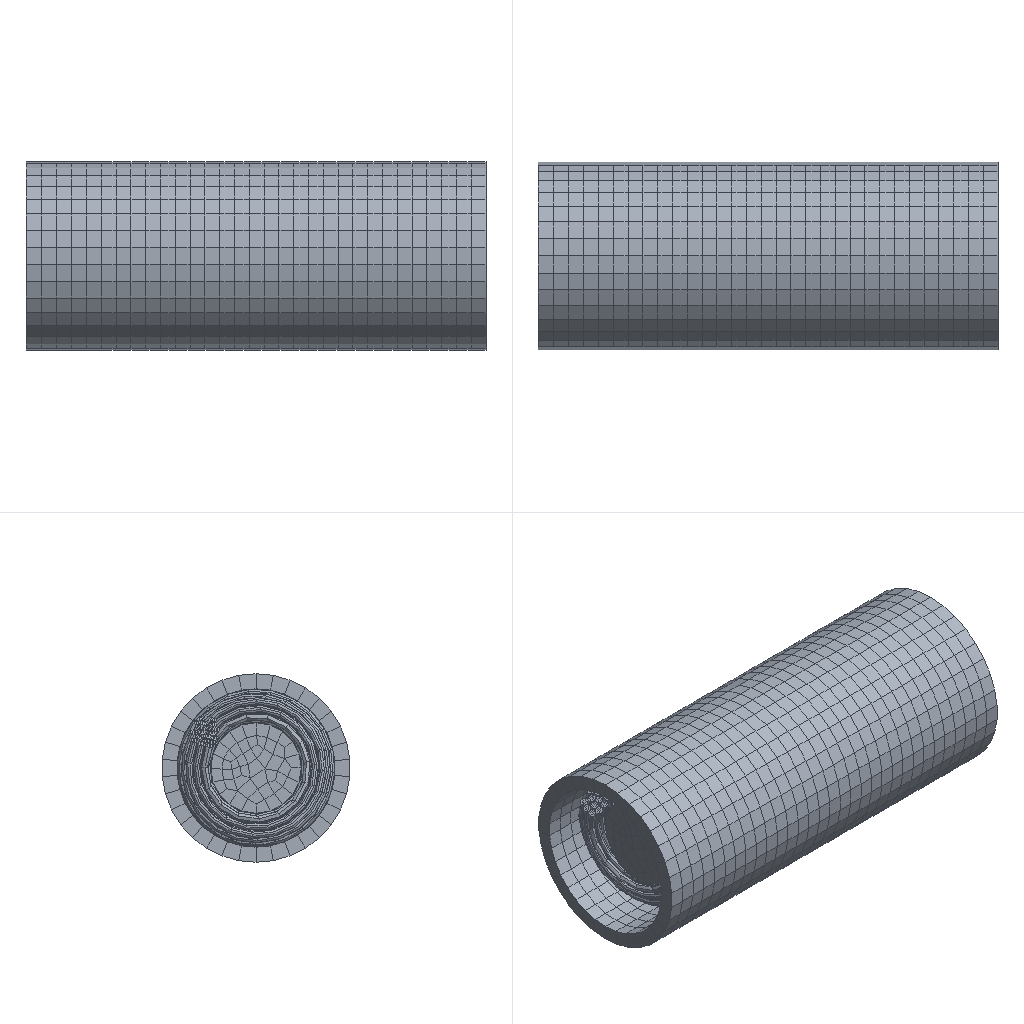Simulation study | abaqus
Set-up summary:
category,name,step,type,value,unit,region
solver,abaqus
solver,version,,,Abaqus/Explicit 2020
units,not stated in the deck,,not stated
analysis,deck,,transient,transient
load_step,Step-1,Step-1,transient,nlgeom=True
contact,interactions,,,general=1 pairs=0 ties=1
load_step,requested,,,1
mesh,nodes,,,49168
mesh,elements,,,34114
element_type,C3D8R,,solid,34114
load,load commands in deck,,count,5
bc,support commands in deck,,count,4
material,MATERIAL-1,,in results
material,TANXIN,,in results
check,setup vs results,,match,"per instance, exact: element labels, types and connectivity; labels of the nodes the elements use; coordinates of those nodes at SINGLE_PRECISION in 2 of 3 instance(s)"
Abaqus input file, long lists of numbers shortened:
*Heading
** Job name: Job-2 Model name: Model-1-Copy
** Generated by: Abaqus/CAE 2020
*Preprint, echo=NO, model=NO, history=NO, contact=NO
**
** PARTS
**
*Part, name=work-2
*Node
      1,          -1.,           0.,   1.05
      2,          -1.,           0.,         1.25
** (2174 more lines like these left out)
*Element, type=C3D8R
  1,   14,   15,    2,    1,  737,  286,   85,  117
  2,   13,   16,   15,   14,  738,  285,  286,  737
** (1052 more lines like these left out)
*Nset, nset=Set-1, generate
    1,  2176,     1
*Elset, elset=Set-1, generate
    1,  1054,     1
** Section: xw
*Solid Section, elset=Set-1, material=Material-1
,
*End Part
**
*Part, name=work-22
*Node
      1,           5., -0.1854,  0.5706
      2,           5., -0.3527,  0.4854
** (1532 more lines like these left out)
*Element, type=C3D8R
   1,   63,   64,  104,   81,    4,    5,   45,   22
   2,   62,   63,   81,   80,    3,    4,   22,   21
** (1198 more lines like these left out)
*Nset, nset=Set-1, generate
    1,  1534,     1
*Elset, elset=Set-1, generate
    1,  1200,     1
** Section: tan
*Solid Section, elset=Set-1, material=tanxin
,
*End Part
**
*Part, name=xianwei
*Node
      1, 0.02713,  0.7191,  0.5041
      2,   4.968, -0.8781, 0.01474
** (45456 more lines like these left out)
*Element, type=C3D8R
   1,  2946,  2942,    40,    39, 21740, 21736,  2960,  2959
   2,  2946,  2943,  2941,  2942, 21740, 21737, 21735, 21736
** (31858 more lines like these left out)
*Nset, nset=Set-2, generate
     1,  45458,      1
*Elset, elset=Set-2, generate
     1,  31860,      1
** Section: xw
*Solid Section, elset=Set-2, material=Material-1
,
*End Part
**
**
** ASSEMBLY
**
*Assembly, name=Assembly
**
*Instance, name=work-2-1, part=work-2
         0.4,           0.,           0.
*End Instance
**
*Instance, name=work-22-1, part=work-22
*End Instance
**
*Instance, name=xianwei-1, part=xianwei
*End Instance
**
*Nset, nset=Set-2, instance=work-2-1
   4,   6,   8,   9,  69,  70,  71,  72,  73,  74,  75,  76,  77,  78,  79,  80
  81,  82,  83,  84, 101, 102, 103, 104, 105, 106, 107, 108, 109, 110, 111, 112
** (3 more lines like these left out)
*Elset, elset=Set-2, instance=work-2-1, generate
   31,  1054,    31
*Nset, nset=Set-3, instance=work-22-1
    1,    2,    3,    4,    5,    6,    7,    8,    9,   10,   11,   12,   13,   14,   15,   16
   17,   18,   19,   20,   21,   22,   23,   24,   25,   26,   27,   28,   29,   30,   31,   32
** (6 more lines like these left out)
*Elset, elset=Set-3, instance=work-22-1
    1,    2,    3,    4,    5,    6,    7,    8,    9,   10,   11,   12,   13,   14,   15,   16
   17,   18,   19,   20,   21,   22,   23,   24,   25,   26,   27,   28,   29,   30,   31,   32
** (4 more lines like these left out)
*Nset, nset=Set-4, instance=work-2-1
   1,   2,   7,  10,  85,  86,  87,  88,  89,  90,  91,  92,  93,  94,  95,  96
  97,  98,  99, 100, 117, 118, 119, 120, 121, 122, 123, 124, 125, 126, 127, 128
** (3 more lines like these left out)
*Elset, elset=Set-4, instance=work-2-1, generate
    1,  1024,    31
*Nset, nset=Set-5, instance=work-22-1, generate
 1476,  1534,     1
*Elset, elset=Set-5, instance=work-22-1, generate
 1153,  1200,     1
*Nset, nset=Set-6, instance=work-22-1, generate
  1,  59,   1
*Elset, elset=Set-6, instance=work-22-1, generate
  1,  48,   1
*Elset, elset=_Surf-7_S4, internal, instance=work-2-1, generate
    1,  1054,     1
*Surface, type=ELEMENT, name=Surf-7
_Surf-7_S4, S4
*Elset, elset=_m_Surf-1_S6, internal, instance=work-2-1, generate
    1,  1054,     1
*Surface, type=ELEMENT, name=m_Surf-1
_m_Surf-1_S6, S6
*Elset, elset=_m_Surf-3_S1, internal, instance=xianwei-1
     1,     2,     3,     4,     5,     6,     7,     8,     9,    10,    11,    12,  1753,  1754,  1755,  1756
  1757,  1758,  1759,  1760,  1761,  1762,  1763,  1764,  3289,  3290,  3291,  3292,  3293,  3294,  3295,  3296
** (12 more lines like these left out)
*Elset, elset=_m_Surf-3_S2, internal, instance=xianwei-1, generate
 16825,  16836,      1
*Surface, type=ELEMENT, name=m_Surf-3
_m_Surf-3_S1, S1
_m_Surf-3_S2, S2
*Elset, elset=_m_Surf-5_S3, internal, instance=work-2-1, generate
   31,  1054,    31
*Surface, type=ELEMENT, name=m_Surf-5
_m_Surf-5_S3, S3
*Elset, elset=_s_Surf-1_S5, internal, instance=xianwei-1
     1,     6,     9,    10,    13,    18,    21,    22,    25,    30,    33,    34,    37,    42,    45,    46
    49,    54,    57,    58,    61,    66,    69,    70,    73,    78,    81,    82,    85,    90,    93,    94
** (662 more lines like these left out)
*Elset, elset=_s_Surf-1_S4, internal, instance=xianwei-1
     3,     5,     8,    12,    15,    17,    20,    24,    27,    29,    32,    36,    39,    41,    44,    48
    51,    53,    56,    60,    63,    65,    68,    72,    75,    77,    80,    84,    87,    89,    92,    96
** (662 more lines like these left out)
*Surface, type=ELEMENT, name=s_Surf-1
_s_Surf-1_S5, S5
_s_Surf-1_S4, S4
*Elset, elset=_s_Surf-5_S2, internal, instance=xianwei-1
  1741,  1742,  1743,  1744,  1745,  1746,  1747,  1748,  1749,  1750,  1751,  1752,  3277,  3278,  3279,  3280
  3281,  3282,  3283,  3284,  3285,  3286,  3287,  3288,  5281,  5282,  5283,  5284,  5285,  5286,  5287,  5288
** (12 more lines like these left out)
*Elset, elset=_s_Surf-5_S1, internal, instance=xianwei-1, generate
 14953,  14964,      1
*Surface, type=ELEMENT, name=s_Surf-5
_s_Surf-5_S2, S2
_s_Surf-5_S1, S1
** Constraint: Constraint-1
*Tie, name=Constraint-1, adjust=yes
s_Surf-1, m_Surf-1
*End Assembly
*Amplitude, name=Amp-1
             0.,              0.,            0.01,              1.
**
** MATERIALS
**
*Material, name=Material-1
*Density
 1.2e-09,
*Elastic
5., 0.35
*Material, name=tanxin
*Density
 2e-09,
*Elastic
10., 0.37
**
** INTERACTION PROPERTIES
**
*Surface Interaction, name=IntProp-1
*Friction
 0.1,
*Surface Behavior, pressure-overclosure=HARD
**
** INTERACTIONS
**
** Interaction: Int-1
*Contact, op=NEW
*Contact Inclusions, ALL EXTERIOR
*Contact Property Assignment
 ,  , IntProp-1
** ----------------------------------------------------------------
**
** STEP: Step-1
**
*Step, name=Step-1, nlgeom=YES
*Dynamic, Explicit
, 0.01
*Bulk Viscosity
0.06, 1.2
** Mass Scaling: Semi-Automatic
**               Whole Model
*Fixed Mass Scaling, factor=50.
**
** BOUNDARY CONDITIONS
**
** Name: BC-1 Type: 位移/转角
*Boundary, amplitude=Amp-1
Set-4, 1, 1, -3.
** Name: BC-2 Type: 位移/转角
*Boundary, amplitude=Amp-1
Set-2, 1, 1, 3.
** Name: BC-4 Type: 位移/转角
*Boundary, amplitude=Amp-1
Set-5, 1, 1, -2.5
** Name: BC-5 Type: 位移/转角
*Boundary, amplitude=Amp-1
Set-6, 1, 1, 2.5
**
** LOADS
**
** Name: Load-1   Type: Pressure
*Dsload, amplitude=Amp-1
Surf-7, P, 0.002
**
** OUTPUT REQUESTS
**
*Restart, write, number interval=1, time marks=NO
**
** FIELD OUTPUT: F-Output-1
**
*Output, field
*Node Output
CF, RF, RM, RT, U, V
*Element Output, directions=YES
E, LE, MISES, MISESMAX, MISESONLY, NE, P, PE, PEEQ, PEEQMAX, PEEQT, PEMAG, PRESSONLY, S, SEQUT, SF
SSAVG, YIELDPOT
*Contact Output
CDISP, CFORCE, CSTRESS, PPRESS
**
** HISTORY OUTPUT: H-Output-1
**
*Output, history, variable=PRESELECT, frequency=1
*End Step
Results summary:
result,step,Step-1,completed,increments=8009 time=0.01/0.01
result,analysis,,,transient
result,last_loadstep,,,1
result,analysis steps,,count,1
result,primary field,,,U
result,reaction total,,FX,-0.001851,model units
result,reaction total,,FY,0.0,model units
result,reaction total,,FZ,0.0,model units